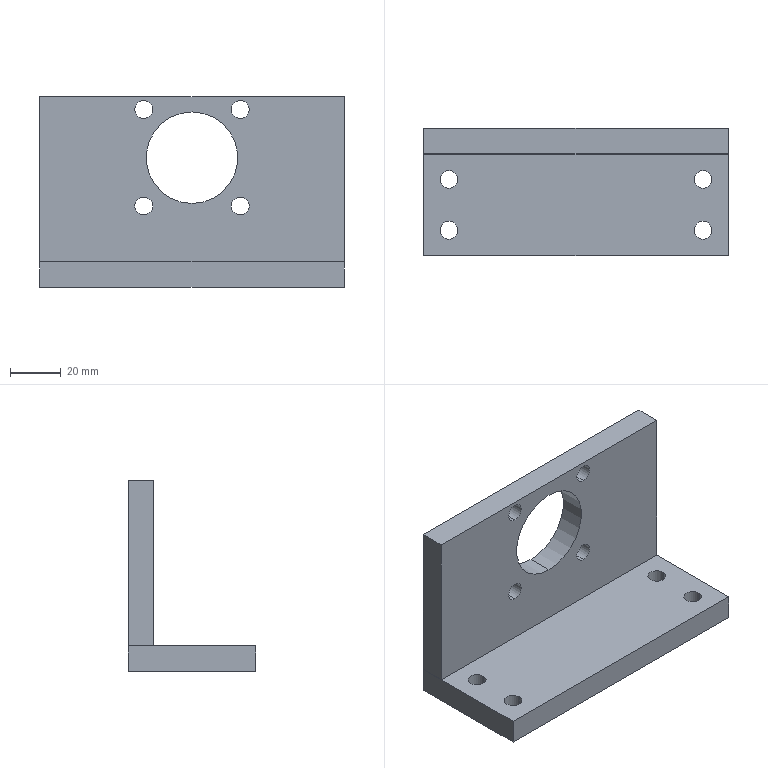Part | STEP file | 44-02-03 Cylinder Mounting Kit | 2 solids | 30 faces | box 120 x 50 x 75 mm | volume 124742 mm3 | cylinder 18 | plane 12 | commonest cylinder face diameters 7 x16 36 x2